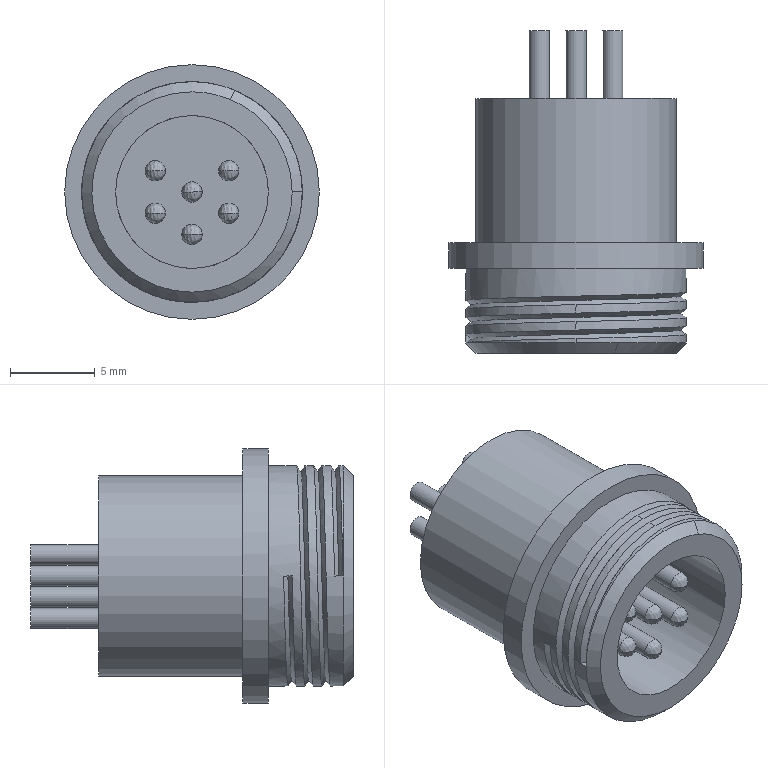Part | NX | 1 solid | 50 faces | box 15 x 19 x 15 mm | volume 1091 mm3 | cylinder 20 | plane 14 | spline 14 | cone 2 | commonest cylinder face diameters 1.2 x12 13 x4 9 x2 11.8 x1 15 x1